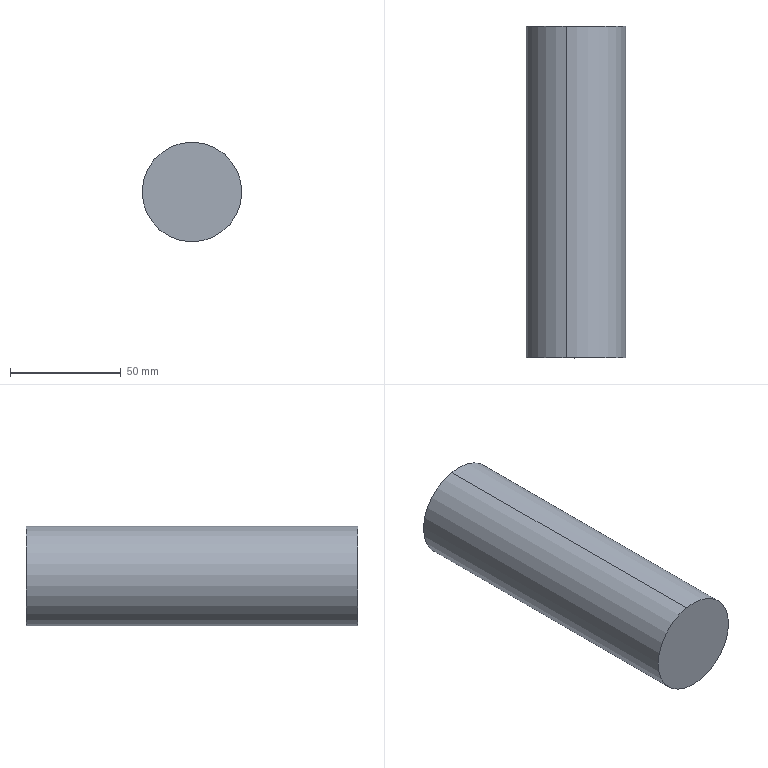Part | STEP file | Boss-Extrude 1-4 | 1 solid | 4 faces | box 45 x 150 x 45 mm | volume 238565 mm3 | cylinder 2 | plane 2 | commonest cylinder face diameters 45 x2
STEP:
#1=CARTESIAN_POINT('',(-744.441,1814.418,3150.28));
#2=VERTEX_POINT('',#1);
#3=CARTESIAN_POINT('',(-753.277,1814.418,3194.404));
#4=VERTEX_POINT('',#3);
#5=CARTESIAN_POINT('',(-748.859,1814.418,3172.342));
#6=DIRECTION('',(0.,-1.,0.));
#7=DIRECTION('',(0.1963,0.,-0.9805));
#8=AXIS2_PLACEMENT_3D('',#5,#6,#7);
#9=CIRCLE('',#8,22.5);
#10=EDGE_CURVE('',#2,#4,#9,.T.);
#11=ORIENTED_EDGE('',*,*,#10,.F.);
#12=CARTESIAN_POINT('',(-744.441,1964.418,3150.28));
#13=VERTEX_POINT('',#12);
#14=CARTESIAN_POINT('',(-744.441,1814.418,3150.28));
#15=DIRECTION('',(0.,-1.,0.));
#16=VECTOR('',#15,1000.);
#17=LINE('',#14,#16);
#18=EDGE_CURVE('',#13,#2,#17,.T.);
#19=ORIENTED_EDGE('',*,*,#18,.F.);
#20=CARTESIAN_POINT('',(-753.277,1964.418,3194.404));
#21=VERTEX_POINT('',#20);
#22=CARTESIAN_POINT('',(-748.859,1964.418,3172.342));
#23=DIRECTION('',(0.,-1.,0.));
#24=DIRECTION('',(0.1963,0.,-0.9805));
#25=AXIS2_PLACEMENT_3D('',#22,#23,#24);
#26=CIRCLE('',#25,22.5);
#27=EDGE_CURVE('',#13,#21,#26,.T.);
#28=ORIENTED_EDGE('',*,*,#27,.T.);
#29=CARTESIAN_POINT('',(-753.277,1814.418,3194.404));
#30=DIRECTION('',(0.,-1.,0.));
#31=VECTOR('',#30,1000.);
#32=LINE('',#29,#31);
#33=EDGE_CURVE('',#21,#4,#32,.T.);
#34=ORIENTED_EDGE('',*,*,#33,.T.);
#35=EDGE_LOOP('',(#11,#19,#28,#34));
#36=FACE_OUTER_BOUND('',#35,.T.);
#37=CARTESIAN_POINT('',(-748.859,1814.418,3172.342));
#38=DIRECTION('',(0.,1.,0.));
#39=DIRECTION('',(0.1963,0.,-0.9805));
#40=AXIS2_PLACEMENT_3D('',#37,#38,#39);
#41=CYLINDRICAL_SURFACE('',#40,22.5);
#42=ADVANCED_FACE('',(#36),#41,.T.);
#43=ORIENTED_EDGE('',*,*,#18,.T.);
#44=CARTESIAN_POINT('',(-748.859,1814.418,3172.342));
#45=DIRECTION('',(0.,-1.,0.));
#46=DIRECTION('',(0.1963,0.,-0.9805));
#47=AXIS2_PLACEMENT_3D('',#44,#45,#46);
#48=CIRCLE('',#47,22.5);
#49=EDGE_CURVE('',#4,#2,#48,.T.);
#50=ORIENTED_EDGE('',*,*,#49,.F.);
#51=ORIENTED_EDGE('',*,*,#33,.F.);
#52=CARTESIAN_POINT('',(-748.859,1964.418,3172.342));
#53=DIRECTION('',(0.,-1.,0.));
#54=DIRECTION('',(0.1963,0.,-0.9805));
#55=AXIS2_PLACEMENT_3D('',#52,#53,#54);
#56=CIRCLE('',#55,22.5);
#57=EDGE_CURVE('',#21,#13,#56,.T.);
#58=ORIENTED_EDGE('',*,*,#57,.T.);
#59=EDGE_LOOP('',(#43,#50,#51,#58));
#60=FACE_OUTER_BOUND('',#59,.T.);
#61=CARTESIAN_POINT('',(-748.859,1814.418,3172.342));
#62=DIRECTION('',(0.,1.,0.));
#63=DIRECTION('',(0.1963,0.,-0.9805));
#64=AXIS2_PLACEMENT_3D('',#61,#62,#63);
#65=CYLINDRICAL_SURFACE('',#64,22.5);
#66=ADVANCED_FACE('',(#60),#65,.T.);
#67=ORIENTED_EDGE('',*,*,#49,.T.);
#68=ORIENTED_EDGE('',*,*,#10,.T.);
#69=EDGE_LOOP('',(#67,#68));
#70=FACE_OUTER_BOUND('',#69,.T.);
#71=CARTESIAN_POINT('',(-748.859,1814.418,3172.342));
#72=DIRECTION('',(0.,-1.,0.));
#73=DIRECTION('',(-0.1963,0.,0.9805));
#74=AXIS2_PLACEMENT_3D('',#71,#72,#73);
#75=PLANE('',#74);
#76=ADVANCED_FACE('',(#70),#75,.T.);
#77=ORIENTED_EDGE('',*,*,#57,.F.);
#78=ORIENTED_EDGE('',*,*,#27,.F.);
#79=EDGE_LOOP('',(#77,#78));
#80=FACE_OUTER_BOUND('',#79,.T.);
#81=CARTESIAN_POINT('',(-748.859,1964.418,3172.342));
#82=DIRECTION('',(0.,-1.,0.));
#83=DIRECTION('',(-0.1963,0.,0.9805));
#84=AXIS2_PLACEMENT_3D('',#81,#82,#83);
#85=PLANE('',#84);
#86=ADVANCED_FACE('',(#80),#85,.F.);
#87=CLOSED_SHELL('',(#42,#66,#76,#86));
#88=MANIFOLD_SOLID_BREP('',#87);
#89=CARTESIAN_POINT('',(0.,0.,0.));
#90=DIRECTION('',(0.,0.,1.));
#91=DIRECTION('',(1.,0.,0.));
#92=AXIS2_PLACEMENT_3D('',#89,#90,#91);
#93=(LENGTH_UNIT()NAMED_UNIT(*)SI_UNIT(.MILLI.,.METRE.));
#94=UNCERTAINTY_MEASURE_WITH_UNIT(LENGTH_MEASURE(0.00001),#93,'','');
#95=(NAMED_UNIT(*)PLANE_ANGLE_UNIT()SI_UNIT($,.RADIAN.));
#96=(NAMED_UNIT(*)SI_UNIT($,.STERADIAN.)SOLID_ANGLE_UNIT());
#97=(GEOMETRIC_REPRESENTATION_CONTEXT(3)GLOBAL_UNCERTAINTY_ASSIGNED_CONTEXT((#94))GLOBAL_UNIT_ASSIGNED_CONTEXT((#93,#95,#96))REPRESENTATION_CONTEXT('',''));
#98=ADVANCED_BREP_SHAPE_REPRESENTATION('',(#88,#92),#97);